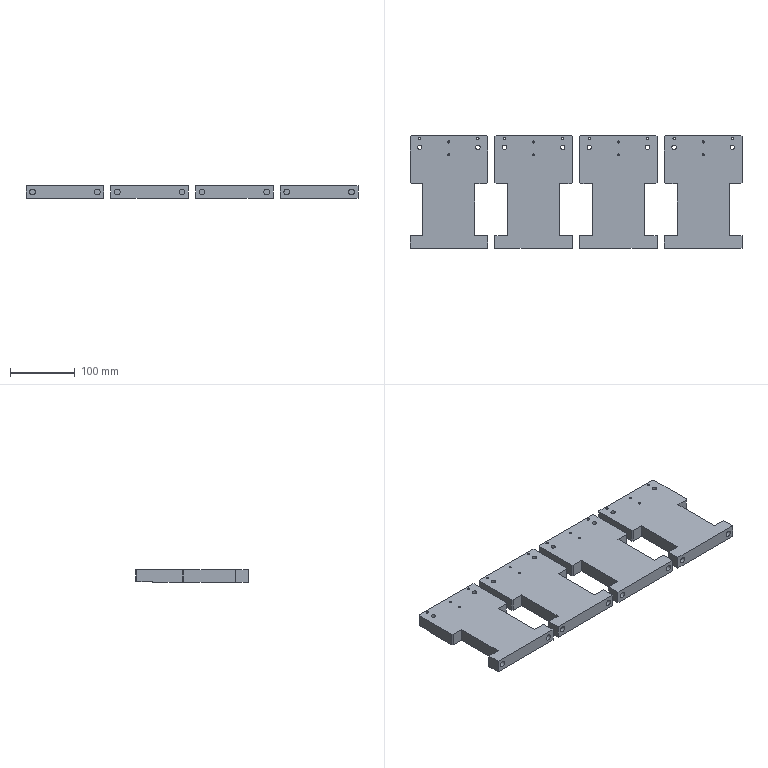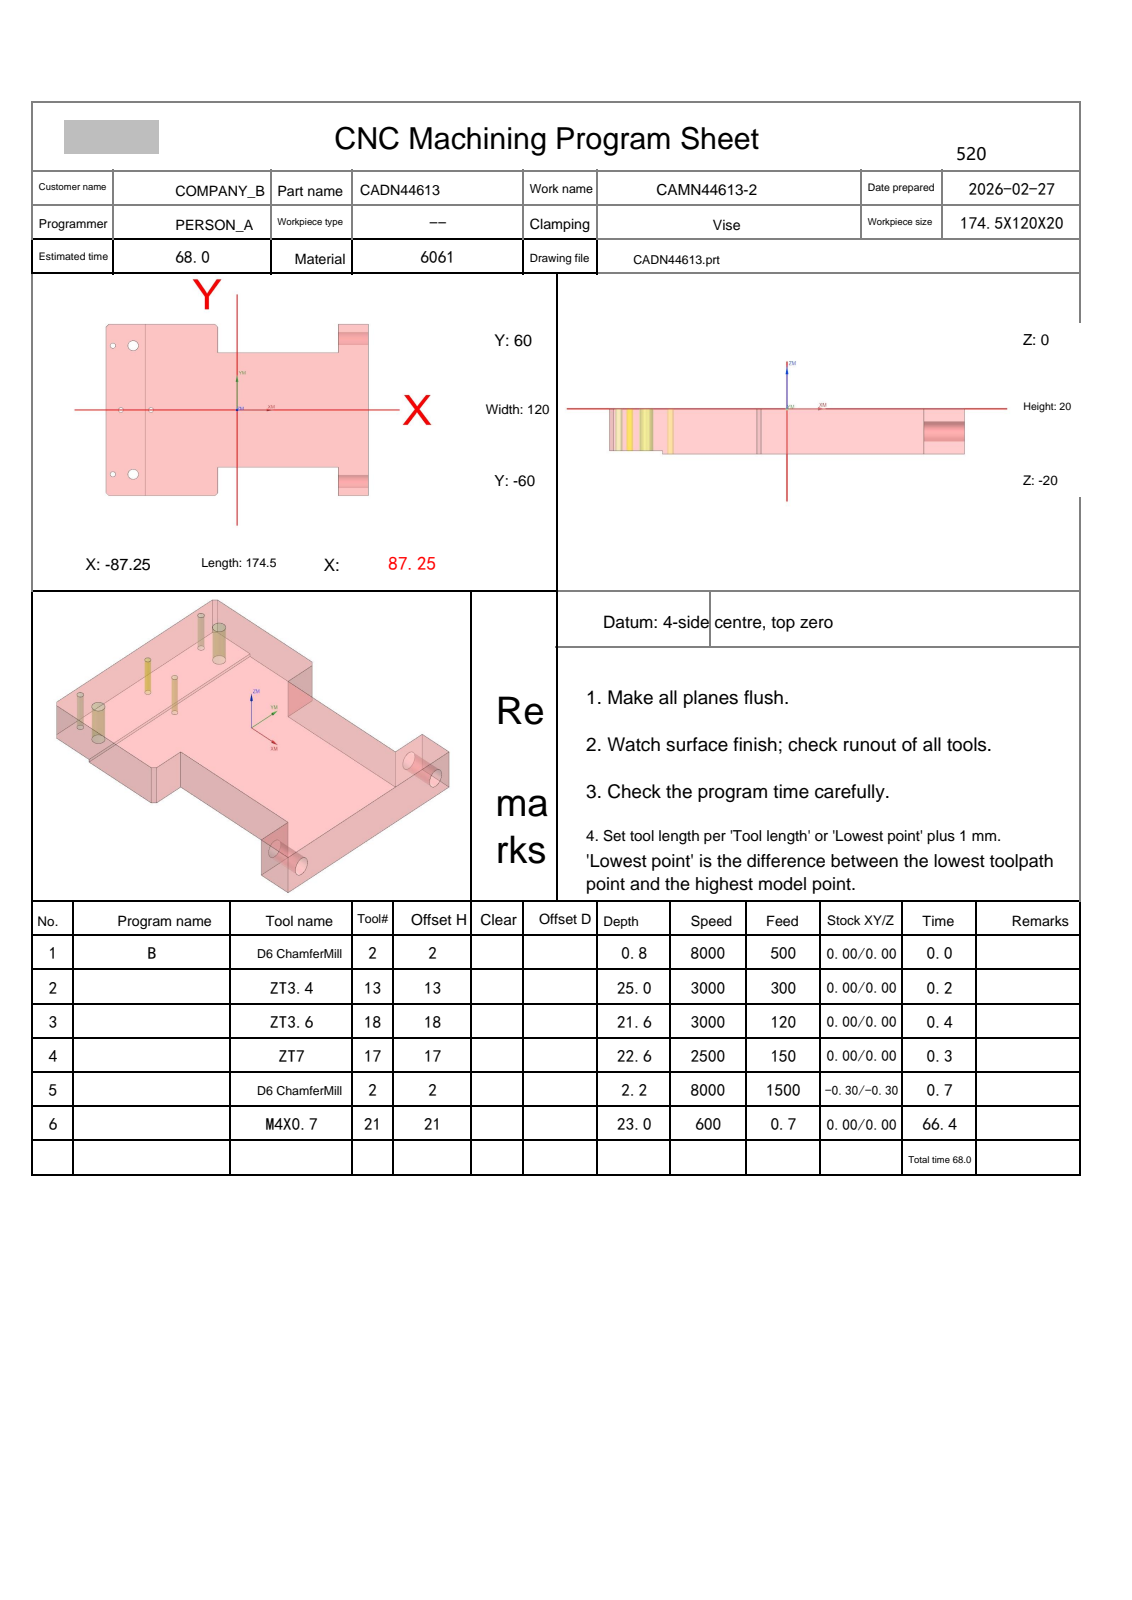NC program | NX | posted by the shop | part box 513 x 174.5 x 20 mm
Whole program:
%
O0001
(Machine time: 132.83 MIN)
(===Total Tool:5===)
(T2=D6 ChamferMill   D=6.   R=0.   D-  H02 Z=-2.2  )
(T13=ZT3.4  D=3.4  DR_a=118 D-  H13 Z=-25.  )
(T18=ZT3.6  D=3.6  DR_a=118 D-  H18 Z=-21.58)
(T17=ZT7    D=7.   DR_a=118 D-  H17 Z=-22.6 )
(T21=M4X0.7 D=3.3  DR_a=180 D-  H21 Z=-23.  )
G80 G90 G17 G49 G40
G91 G28 Z0
M01
N1 T02 M06
(D6 ChamferMill  D=6. R=0. H=02 ce=0.00 di=0.00)
G00 G90 G54 X-82.6 Y-45. M03 S8000
G43 H02 Z30.
M08
G98 G81 X-82.6 Y-45. Z-.8 R1. F500.
X-69.1
X-57.25 Y0.0
X-77.25
X-82.6 Y45.
X-69.1
G80
G00 Z30.
G91 G28 Z0.0
M05
M09
G91 G28 Z0.0
M01
N2 T13 M06
(ZT3.4 D=3.4 DR_a=118 H=13)
G00 G90 G54 X-77.25 Y0.0 M03 S3000
G43 H13 Z30.
M08
G98 G83 X-77.25 Y0.0 Z-25. R1. F300. Q2.
X-57.25
G80
G00 Z30.
G91 G28 Z0.0
M05
M09
G91 G28 Z0.0
M01
N3 T18 M06
(ZT3.6 D=3.6 DR_a=118 H=18)
G00 G90 G54 X-82.6 Y-45. M03 S3000
G43 H18 Z30.
M08
G98 G83 X-82.6 Y-45. Z-21.582 R1. F120. Q3.
Y45.
G80
G00 Z30.
G91 G28 Z0.0
M05
M09
G91 G28 Z0.0
M01
N4 T17 M06
(ZT7 D=7. DR_a=118 H=17)
G00 G90 G54 X-69.1 Y45. M03 S2500
G43 H17 Z30.
M08
G98 G83 X-69.1 Y45. Z-22.603 R1. F150. Q3.
Y-45.
G80
G00 Z30.
G91 G28 Z0.0
M05
M09
G91 G28 Z0.0
M01
N5 T02 M06
(D6 ChamferMill  D=6. R=0. H=02 ce=0.00 di=0.00)
G00 G90 G54 X-77.25 Y0.0 M03 S8000
G43 H02 Z30.
M08
G98 G81 X-77.25 Y0.0 Z-2.2 R3. F500.
X-57.25
G80
G00 Z30.
G00 G90 X-82.6 Y-45. M03 S8000
Z30.
G98 G81 X-82.6 Y-45. Z-2.1 R3. F500.
Y45.
G80
G00 Z30.
G00 G90 X-70.6 Y44.005 M03 S8000
Z30.
Z-.5
G01 Z-1. F800.
Y43.7
G03 X-69.1 Y42.2 I1.5 J0.0
X-66.3 Y45. I0.0 J2.8
X-69.1 Y47.8 I-2.8 J0.0
X-71.9 Y45. I0.0 J-2.8
X-69.1 Y42.2 I2.8 J0.0
X-67.6 Y43.7 I0.0 J1.5
G01 Y44.005
Z-.5
G00 Z30.
X-70.6 Y-45.995
Z-.5
G01 Z-1.
Y-46.3
G03 X-69.1 Y-47.8 I1.5 J0.0
X-66.3 Y-45. I0.0 J2.8
X-69.1 Y-42.2 I-2.8 J0.0
X-71.9 Y-45. I0.0 J-2.8
X-69.1 Y-47.8 I2.8 J0.0
X-67.6 Y-46.3 I0.0 J1.5
G01 Y-45.995
Z-.5
G00 Z30.
G00 G90 X88.377 Y.386 M03 S8000
Z30.
Z.272
G01 Z-1.2 F1500.
G03 X88.177 Y.1 I1.532 J-1.286
G01 X88.147 Y.054
X88.15 Y0.0
Y-60.
G02 X87.25 Y-60.9 I-.9 J0.0
G01 X67.25
G02 X66.35 Y-60. I0.0 J.9
G01 Y-40.9
X-11.85
Y-58.
X-11.881 Y-58.233
X-11.971 Y-58.45
X-12.114 Y-58.636
X-14.114 Y-60.636
X-14.3 Y-60.779
X-14.517 Y-60.869
X-14.75 Y-60.9
X-85.25
X-85.483 Y-60.869
X-85.7 Y-60.779
X-85.886 Y-60.636
X-87.886 Y-58.636
X-88.029 Y-58.45
X-88.119 Y-58.233
X-88.15 Y-58.
Y58.
X-88.119 Y58.233
X-88.029 Y58.45
X-87.886 Y58.636
X-85.886 Y60.636
X-85.7 Y60.779
X-85.483 Y60.869
X-85.25 Y60.9
X-14.75
X-14.517 Y60.869
X-14.3 Y60.779
X-14.114 Y60.636
X-12.114 Y58.636
X-11.971 Y58.45
X-11.881 Y58.233
X-11.85 Y58.
Y40.9
X66.35
Y60.
G02 X67.25 Y60.9 I.9 J0.0
G01 X87.25
G02 X88.15 Y60. I0.0 J-.9
G01 Y0.0
X88.147 Y-.054
X88.177 Y-.1
G03 X88.377 Y-.386 I1.732 J1.
G01 Z.272
G00 Z10.
X-69.504 Y42.592
Z.346
G01 Z-1.2
G03 X-69.202 Y42.418 I1.147 J1.638
G01 X-69.154 Y42.392
X-69.1 Y42.4
G03 X-66.5 Y45. I0.0 J2.6
X-69.1 Y47.6 I-2.6 J0.0
X-71.7 Y45. I0.0 J-2.6
X-69.1 Y42.4 I2.6 J0.0
G01 X-69.046 Y42.392
X-68.998 Y42.418
G03 X-68.696 Y42.592 I-.845 J1.813
G01 Z.346
G00 Z10.
X-83.012 Y44.274
Z.443
G01 Z-1.2
G03 X-82.703 Y44.114 I1.075 J1.687
G01 X-82.654 Y44.09
X-82.6 Y44.1
G03 X-81.7 Y45. I0.0 J.9
X-82.6 Y45.9 I-.9 J0.0
X-83.5 Y45. I0.0 J-.9
X-82.6 Y44.1 I.9 J0.0
G01 X-82.546 Y44.09
X-82.497 Y44.114
G03 X-82.188 Y44.274 I-.765 J1.848
G01 Z.443
G00 Z10.
X-77.662 Y-.576
Z.466
G01 Z-1.2
G03 X-77.353 Y-.736 I1.075 J1.687
G01 X-77.304 Y-.76
X-77.25 Y-.75
G03 X-76.5 Y0.0 I0.0 J.75
X-77.25 Y.75 I-.75 J0.0
X-78. Y0.0 I0.0 J-.75
X-77.444 Y-.724 I.75 J0.0
G01 X-77.25 Y-.75
X-77.196 Y-.76
X-77.147 Y-.736
G03 X-76.838 Y-.576 I-.765 J1.848
G01 Z.466
G00 Z10.
X-57.662
Z.466
G01 Z-1.2
G03 X-57.353 Y-.736 I1.075 J1.687
G01 X-57.304 Y-.76
X-57.25 Y-.75
G03 X-56.5 Y0.0 I0.0 J.75
X-57.25 Y.75 I-.75 J0.0
X-58. Y0.0 I0.0 J-.75
X-57.444 Y-.724 I.75 J0.0
G01 X-57.25 Y-.75
X-57.196 Y-.76
X-57.147 Y-.736
G03 X-56.838 Y-.576 I-.765 J1.848
G01 Z.466
G00 Z10.
X-69.504 Y-47.408
Z.346
G01 Z-1.2
G03 X-69.202 Y-47.582 I1.147 J1.638
G01 X-69.154 Y-47.608
X-69.1 Y-47.6
G03 X-66.5 Y-45. I0.0 J2.6
X-69.1 Y-42.4 I-2.6 J0.0
X-71.7 Y-45. I0.0 J-2.6
X-69.1 Y-47.6 I2.6 J0.0
G01 X-69.046 Y-47.608
X-68.998 Y-47.582
G03 X-68.696 Y-47.408 I-.845 J1.813
G01 Z.346
G00 Z10.
X-83.012 Y-45.726
Z.443
G01 Z-1.2
G03 X-82.703 Y-45.886 I1.075 J1.687
G01 X-82.654 Y-45.91
X-82.6 Y-45.9
G03 X-81.7 Y-45. I0.0 J.9
X-82.6 Y-44.1 I-.9 J0.0
X-83.5 Y-45. I0.0 J-.9
X-82.6 Y-45.9 I.9 J0.0
G01 X-82.546 Y-45.91
X-82.497 Y-45.886
G03 X-82.188 Y-45.726 I-.765 J1.848
G01 Z.443
G00 Z30.
G91 G28 Z0.0
M05
M09
G91 G28 Z0.0
M01
N6 T21 M06
(M4X0.7 D=3.3 DR_a=180 H=21)
G00 G90 G54 X-77.25 Y0.0 M03 S600
G43 H21 Z30.
M08
G95
G98 G84 X-77.25 Y0.0 Z-21.5 R1. F.7 Q4.
G98 G84 X-57.25 Y0.0 Z-23. R1.
G80
G94
G00 Z30.
M05
M09
G91 G28 Z0.0
G91 G28 Y0.0
M30
%